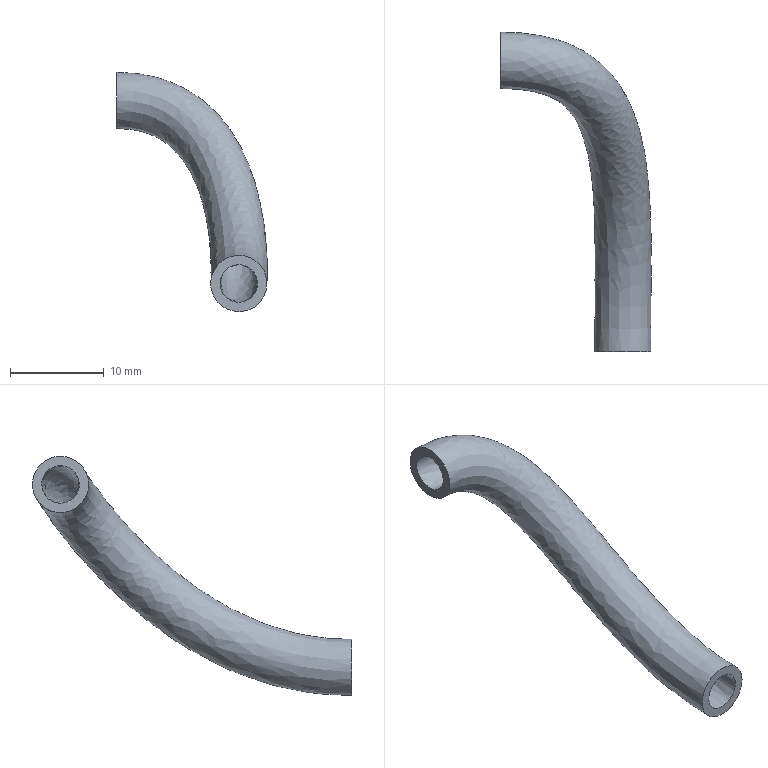Part | NX | features solid 2 | 1 solid | 4 faces | box 16.038 x 34.023 x 25.5 mm | volume 701.534 mm3 | plane 2 | spline 2